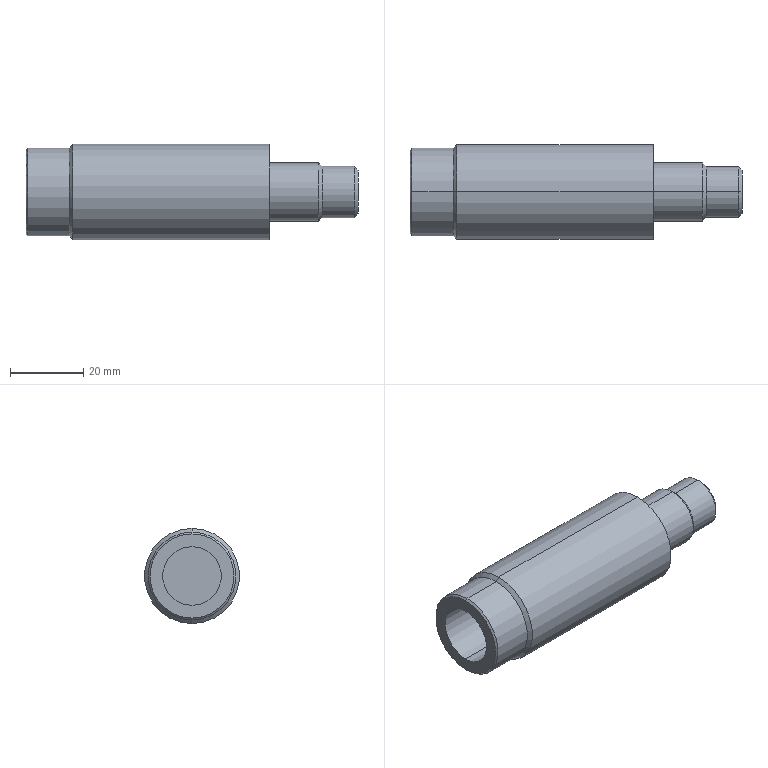Part | SolidWorks | features Chamfer 3, Revolution 1 | 1 solid | 22 faces | box 90.69 x 26 x 26 mm | volume 34532 mm3 | cylinder 10 | cone 8 | plane 4 | commonest cylinder face diameters 16 x4 14 x2 24 x2 26 x2
STEP:
#1=CARTESIAN_POINT('',(-33.026,0.,11.5));
#2=VERTEX_POINT('',#1);
#3=CARTESIAN_POINT('',(-33.026,0.,-11.5));
#4=VERTEX_POINT('',#3);
#5=CARTESIAN_POINT('',(-33.026,0.,0.));
#6=DIRECTION('',(-1.,0.,0.));
#7=DIRECTION('',(0.,0.,-1.));
#8=AXIS2_PLACEMENT_3D('',#5,#6,#7);
#9=CIRCLE('',#8,11.5);
#10=EDGE_CURVE('',#2,#4,#9,.T.);
#11=ORIENTED_EDGE('',*,*,#10,.F.);
#12=CARTESIAN_POINT('',(-32.526,0.,12.));
#13=VERTEX_POINT('',#12);
#14=CARTESIAN_POINT('',(-33.026,0.,11.5));
#15=DIRECTION('',(0.7071,0.,0.7071));
#16=VECTOR('',#15,1000.);
#17=LINE('',#14,#16);
#18=EDGE_CURVE('',#2,#13,#17,.T.);
#19=ORIENTED_EDGE('',*,*,#18,.T.);
#20=CARTESIAN_POINT('',(-32.526,0.,-12.));
#21=VERTEX_POINT('',#20);
#22=CARTESIAN_POINT('',(-32.526,0.,0.));
#23=DIRECTION('',(1.,0.,0.));
#24=DIRECTION('',(0.,0.,-1.));
#25=AXIS2_PLACEMENT_3D('',#22,#23,#24);
#26=CIRCLE('',#25,12.);
#27=EDGE_CURVE('',#21,#13,#26,.T.);
#28=ORIENTED_EDGE('',*,*,#27,.F.);
#29=CARTESIAN_POINT('',(-33.026,0.,-11.5));
#30=DIRECTION('',(0.7071,0.,-0.7071));
#31=VECTOR('',#30,1000.);
#32=LINE('',#29,#31);
#33=EDGE_CURVE('',#4,#21,#32,.T.);
#34=ORIENTED_EDGE('',*,*,#33,.F.);
#35=EDGE_LOOP('',(#11,#19,#28,#34));
#36=FACE_OUTER_BOUND('',#35,.T.);
#37=CARTESIAN_POINT('',(-33.026,0.,0.));
#38=DIRECTION('',(1.,0.,0.));
#39=DIRECTION('',(0.,0.,-1.));
#40=AXIS2_PLACEMENT_3D('',#37,#38,#39);
#41=CONICAL_SURFACE('',#40,11.5,0.7854);
#42=ADVANCED_FACE('',(#36),#41,.T.);
#43=CARTESIAN_POINT('',(47.874,0.,7.));
#44=VERTEX_POINT('',#43);
#45=CARTESIAN_POINT('',(47.874,0.,-7.));
#46=VERTEX_POINT('',#45);
#47=CARTESIAN_POINT('',(47.874,0.,0.));
#48=DIRECTION('',(-1.,0.,0.));
#49=DIRECTION('',(0.,0.,1.));
#50=AXIS2_PLACEMENT_3D('',#47,#48,#49);
#51=CIRCLE('',#50,7.);
#52=EDGE_CURVE('',#44,#46,#51,.T.);
#53=ORIENTED_EDGE('',*,*,#52,.T.);
#54=CARTESIAN_POINT('',(46.874,0.,-8.));
#55=VERTEX_POINT('',#54);
#56=CARTESIAN_POINT('',(46.874,0.,-8.));
#57=DIRECTION('',(-0.7071,0.,-0.7071));
#58=VECTOR('',#57,1000.);
#59=LINE('',#56,#58);
#60=EDGE_CURVE('',#46,#55,#59,.T.);
#61=ORIENTED_EDGE('',*,*,#60,.T.);
#62=CARTESIAN_POINT('',(46.874,0.,8.));
#63=VERTEX_POINT('',#62);
#64=CARTESIAN_POINT('',(46.874,0.,0.));
#65=DIRECTION('',(-1.,0.,0.));
#66=DIRECTION('',(0.,0.,1.));
#67=AXIS2_PLACEMENT_3D('',#64,#65,#66);
#68=CIRCLE('',#67,8.);
#69=EDGE_CURVE('',#63,#55,#68,.T.);
#70=ORIENTED_EDGE('',*,*,#69,.F.);
#71=CARTESIAN_POINT('',(46.874,0.,8.));
#72=DIRECTION('',(-0.7071,0.,0.7071));
#73=VECTOR('',#72,1000.);
#74=LINE('',#71,#73);
#75=EDGE_CURVE('',#44,#63,#74,.T.);
#76=ORIENTED_EDGE('',*,*,#75,.F.);
#77=EDGE_LOOP('',(#53,#61,#70,#76));
#78=FACE_OUTER_BOUND('',#77,.T.);
#79=CARTESIAN_POINT('',(46.874,0.,0.));
#80=DIRECTION('',(-1.,0.,0.));
#81=DIRECTION('',(0.,0.,1.));
#82=AXIS2_PLACEMENT_3D('',#79,#80,#81);
#83=CONICAL_SURFACE('',#82,8.,0.7854);
#84=ADVANCED_FACE('',(#78),#83,.T.);
#85=CARTESIAN_POINT('',(57.664,0.,-6.));
#86=VERTEX_POINT('',#85);
#87=CARTESIAN_POINT('',(57.664,0.,6.));
#88=VERTEX_POINT('',#87);
#89=CARTESIAN_POINT('',(57.664,0.,0.));
#90=DIRECTION('',(1.,0.,0.));
#91=DIRECTION('',(0.,0.,1.));
#92=AXIS2_PLACEMENT_3D('',#89,#90,#91);
#93=CIRCLE('',#92,6.);
#94=EDGE_CURVE('',#86,#88,#93,.T.);
#95=ORIENTED_EDGE('',*,*,#94,.F.);
#96=CARTESIAN_POINT('',(56.664,0.,-7.));
#97=VERTEX_POINT('',#96);
#98=CARTESIAN_POINT('',(56.664,0.,-7.));
#99=DIRECTION('',(-0.7071,0.,-0.7071));
#100=VECTOR('',#99,1000.);
#101=LINE('',#98,#100);
#102=EDGE_CURVE('',#86,#97,#101,.T.);
#103=ORIENTED_EDGE('',*,*,#102,.T.);
#104=CARTESIAN_POINT('',(56.664,0.,7.));
#105=VERTEX_POINT('',#104);
#106=CARTESIAN_POINT('',(56.664,0.,0.));
#107=DIRECTION('',(-1.,0.,0.));
#108=DIRECTION('',(0.,0.,1.));
#109=AXIS2_PLACEMENT_3D('',#106,#107,#108);
#110=CIRCLE('',#109,7.);
#111=EDGE_CURVE('',#105,#97,#110,.T.);
#112=ORIENTED_EDGE('',*,*,#111,.F.);
#113=CARTESIAN_POINT('',(56.664,0.,7.));
#114=DIRECTION('',(-0.7071,0.,0.7071));
#115=VECTOR('',#114,1000.);
#116=LINE('',#113,#115);
#117=EDGE_CURVE('',#88,#105,#116,.T.);
#118=ORIENTED_EDGE('',*,*,#117,.F.);
#119=EDGE_LOOP('',(#95,#103,#112,#118));
#120=FACE_OUTER_BOUND('',#119,.T.);
#121=CARTESIAN_POINT('',(56.664,0.,0.));
#122=DIRECTION('',(-1.,0.,0.));
#123=DIRECTION('',(0.,0.,1.));
#124=AXIS2_PLACEMENT_3D('',#121,#122,#123);
#125=CONICAL_SURFACE('',#124,7.,0.7854);
#126=ADVANCED_FACE('',(#120),#125,.T.);
#127=CARTESIAN_POINT('',(-21.21,0.,12.));
#128=VERTEX_POINT('',#127);
#129=CARTESIAN_POINT('',(-21.21,0.,-12.));
#130=VERTEX_POINT('',#129);
#131=CARTESIAN_POINT('',(-21.21,0.,0.));
#132=DIRECTION('',(-1.,0.,0.));
#133=DIRECTION('',(0.,0.,1.));
#134=AXIS2_PLACEMENT_3D('',#131,#132,#133);
#135=CIRCLE('',#134,12.);
#136=EDGE_CURVE('',#128,#130,#135,.T.);
#137=ORIENTED_EDGE('',*,*,#136,.F.);
#138=CARTESIAN_POINT('',(-20.21,0.,13.));
#139=VERTEX_POINT('',#138);
#140=CARTESIAN_POINT('',(-21.21,0.,12.));
#141=DIRECTION('',(0.7071,0.,0.7071));
#142=VECTOR('',#141,1000.);
#143=LINE('',#140,#142);
#144=EDGE_CURVE('',#128,#139,#143,.T.);
#145=ORIENTED_EDGE('',*,*,#144,.T.);
#146=CARTESIAN_POINT('',(-20.21,0.,-13.));
#147=VERTEX_POINT('',#146);
#148=CARTESIAN_POINT('',(-20.21,0.,0.));
#149=DIRECTION('',(1.,0.,0.));
#150=DIRECTION('',(0.,0.,-1.));
#151=AXIS2_PLACEMENT_3D('',#148,#149,#150);
#152=CIRCLE('',#151,13.);
#153=EDGE_CURVE('',#147,#139,#152,.T.);
#154=ORIENTED_EDGE('',*,*,#153,.F.);
#155=CARTESIAN_POINT('',(-21.21,0.,-12.));
#156=DIRECTION('',(0.7071,0.,-0.7071));
#157=VECTOR('',#156,1000.);
#158=LINE('',#155,#157);
#159=EDGE_CURVE('',#130,#147,#158,.T.);
#160=ORIENTED_EDGE('',*,*,#159,.F.);
#161=EDGE_LOOP('',(#137,#145,#154,#160));
#162=FACE_OUTER_BOUND('',#161,.T.);
#163=CARTESIAN_POINT('',(-21.21,0.,0.));
#164=DIRECTION('',(1.,0.,0.));
#165=DIRECTION('',(0.,0.,-1.));
#166=AXIS2_PLACEMENT_3D('',#163,#164,#165);
#167=CONICAL_SURFACE('',#166,12.,0.7854);
#168=ADVANCED_FACE('',(#162),#167,.T.);
#169=ORIENTED_EDGE('',*,*,#111,.T.);
#170=CARTESIAN_POINT('',(-58.891,0.,-7.));
#171=DIRECTION('',(-1.,0.,0.));
#172=VECTOR('',#171,1000.);
#173=LINE('',#170,#172);
#174=EDGE_CURVE('',#97,#46,#173,.T.);
#175=ORIENTED_EDGE('',*,*,#174,.T.);
#176=ORIENTED_EDGE('',*,*,#52,.F.);
#177=CARTESIAN_POINT('',(-58.891,0.,7.));
#178=DIRECTION('',(-1.,0.,0.));
#179=VECTOR('',#178,1000.);
#180=LINE('',#177,#179);
#181=EDGE_CURVE('',#105,#44,#180,.T.);
#182=ORIENTED_EDGE('',*,*,#181,.F.);
#183=EDGE_LOOP('',(#169,#175,#176,#182));
#184=FACE_OUTER_BOUND('',#183,.T.);
#185=CARTESIAN_POINT('',(-58.891,0.,0.));
#186=DIRECTION('',(-1.,0.,0.));
#187=DIRECTION('',(0.,0.,1.));
#188=AXIS2_PLACEMENT_3D('',#185,#186,#187);
#189=CYLINDRICAL_SURFACE('',#188,7.);
#190=ADVANCED_FACE('',(#184),#189,.T.);
#191=ORIENTED_EDGE('',*,*,#69,.T.);
#192=CARTESIAN_POINT('',(33.374,0.,-8.));
#193=VERTEX_POINT('',#192);
#194=CARTESIAN_POINT('',(-58.891,0.,-8.));
#195=DIRECTION('',(-1.,0.,0.));
#196=VECTOR('',#195,1000.);
#197=LINE('',#194,#196);
#198=EDGE_CURVE('',#55,#193,#197,.T.);
#199=ORIENTED_EDGE('',*,*,#198,.T.);
#200=CARTESIAN_POINT('',(33.374,0.,8.));
#201=VERTEX_POINT('',#200);
#202=CARTESIAN_POINT('',(33.374,0.,0.));
#203=DIRECTION('',(-1.,0.,0.));
#204=DIRECTION('',(0.,0.,1.));
#205=AXIS2_PLACEMENT_3D('',#202,#203,#204);
#206=CIRCLE('',#205,8.);
#207=EDGE_CURVE('',#201,#193,#206,.T.);
#208=ORIENTED_EDGE('',*,*,#207,.F.);
#209=CARTESIAN_POINT('',(-58.891,0.,8.));
#210=DIRECTION('',(-1.,0.,0.));
#211=VECTOR('',#210,1000.);
#212=LINE('',#209,#211);
#213=EDGE_CURVE('',#63,#201,#212,.T.);
#214=ORIENTED_EDGE('',*,*,#213,.F.);
#215=EDGE_LOOP('',(#191,#199,#208,#214));
#216=FACE_OUTER_BOUND('',#215,.T.);
#217=CARTESIAN_POINT('',(-58.891,0.,0.));
#218=DIRECTION('',(-1.,0.,0.));
#219=DIRECTION('',(0.,0.,1.));
#220=AXIS2_PLACEMENT_3D('',#217,#218,#219);
#221=CYLINDRICAL_SURFACE('',#220,8.);
#222=ADVANCED_FACE('',(#216),#221,.T.);
#223=CARTESIAN_POINT('',(33.374,0.,13.));
#224=VERTEX_POINT('',#223);
#225=CARTESIAN_POINT('',(33.374,0.,-13.));
#226=VERTEX_POINT('',#225);
#227=CARTESIAN_POINT('',(33.374,0.,0.));
#228=DIRECTION('',(-1.,0.,0.));
#229=DIRECTION('',(0.,0.,1.));
#230=AXIS2_PLACEMENT_3D('',#227,#228,#229);
#231=CIRCLE('',#230,13.);
#232=EDGE_CURVE('',#224,#226,#231,.T.);
#233=ORIENTED_EDGE('',*,*,#232,.T.);
#234=CARTESIAN_POINT('',(-58.891,0.,-13.));
#235=DIRECTION('',(-1.,0.,0.));
#236=VECTOR('',#235,1000.);
#237=LINE('',#234,#236);
#238=EDGE_CURVE('',#226,#147,#237,.T.);
#239=ORIENTED_EDGE('',*,*,#238,.T.);
#240=ORIENTED_EDGE('',*,*,#153,.T.);
#241=CARTESIAN_POINT('',(-58.891,0.,13.));
#242=DIRECTION('',(-1.,0.,0.));
#243=VECTOR('',#242,1000.);
#244=LINE('',#241,#243);
#245=EDGE_CURVE('',#224,#139,#244,.T.);
#246=ORIENTED_EDGE('',*,*,#245,.F.);
#247=EDGE_LOOP('',(#233,#239,#240,#246));
#248=FACE_OUTER_BOUND('',#247,.T.);
#249=CARTESIAN_POINT('',(-58.891,0.,0.));
#250=DIRECTION('',(-1.,0.,0.));
#251=DIRECTION('',(0.,0.,1.));
#252=AXIS2_PLACEMENT_3D('',#249,#250,#251);
#253=CYLINDRICAL_SURFACE('',#252,13.);
#254=ADVANCED_FACE('',(#248),#253,.T.);
#255=ORIENTED_EDGE('',*,*,#136,.T.);
#256=CARTESIAN_POINT('',(-58.891,0.,-12.));
#257=DIRECTION('',(-1.,0.,0.));
#258=VECTOR('',#257,1000.);
#259=LINE('',#256,#258);
#260=EDGE_CURVE('',#130,#21,#259,.T.);
#261=ORIENTED_EDGE('',*,*,#260,.T.);
#262=ORIENTED_EDGE('',*,*,#27,.T.);
#263=CARTESIAN_POINT('',(-58.891,0.,12.));
#264=DIRECTION('',(-1.,0.,0.));
#265=VECTOR('',#264,1000.);
#266=LINE('',#263,#265);
#267=EDGE_CURVE('',#128,#13,#266,.T.);
#268=ORIENTED_EDGE('',*,*,#267,.F.);
#269=EDGE_LOOP('',(#255,#261,#262,#268));
#270=FACE_OUTER_BOUND('',#269,.T.);
#271=CARTESIAN_POINT('',(-58.891,0.,0.));
#272=DIRECTION('',(-1.,0.,0.));
#273=DIRECTION('',(0.,0.,1.));
#274=AXIS2_PLACEMENT_3D('',#271,#272,#273);
#275=CYLINDRICAL_SURFACE('',#274,12.);
#276=ADVANCED_FACE('',(#270),#275,.T.);
#277=CARTESIAN_POINT('',(-12.526,0.,-8.));
#278=VERTEX_POINT('',#277);
#279=CARTESIAN_POINT('',(-12.526,0.,8.));
#280=VERTEX_POINT('',#279);
#281=CARTESIAN_POINT('',(-12.526,0.,0.));
#282=DIRECTION('',(-1.,0.,0.));
#283=DIRECTION('',(0.,0.,1.));
#284=AXIS2_PLACEMENT_3D('',#281,#282,#283);
#285=CIRCLE('',#284,8.);
#286=EDGE_CURVE('',#278,#280,#285,.T.);
#287=ORIENTED_EDGE('',*,*,#286,.F.);
#288=CARTESIAN_POINT('',(-33.026,0.,-8.));
#289=VERTEX_POINT('',#288);
#290=CARTESIAN_POINT('',(-58.891,0.,-8.));
#291=DIRECTION('',(-1.,0.,0.));
#292=VECTOR('',#291,1000.);
#293=LINE('',#290,#292);
#294=EDGE_CURVE('',#278,#289,#293,.T.);
#295=ORIENTED_EDGE('',*,*,#294,.T.);
#296=CARTESIAN_POINT('',(-33.026,0.,8.));
#297=VERTEX_POINT('',#296);
#298=CARTESIAN_POINT('',(-33.026,0.,0.));
#299=DIRECTION('',(-1.,0.,0.));
#300=DIRECTION('',(0.,0.,1.));
#301=AXIS2_PLACEMENT_3D('',#298,#299,#300);
#302=CIRCLE('',#301,8.);
#303=EDGE_CURVE('',#289,#297,#302,.T.);
#304=ORIENTED_EDGE('',*,*,#303,.T.);
#305=CARTESIAN_POINT('',(-58.891,0.,8.));
#306=DIRECTION('',(-1.,0.,0.));
#307=VECTOR('',#306,1000.);
#308=LINE('',#305,#307);
#309=EDGE_CURVE('',#280,#297,#308,.T.);
#310=ORIENTED_EDGE('',*,*,#309,.F.);
#311=EDGE_LOOP('',(#287,#295,#304,#310));
#312=FACE_OUTER_BOUND('',#311,.T.);
#313=CARTESIAN_POINT('',(-58.891,0.,0.));
#314=DIRECTION('',(-1.,0.,0.));
#315=DIRECTION('',(0.,0.,1.));
#316=AXIS2_PLACEMENT_3D('',#313,#314,#315);
#317=CYLINDRICAL_SURFACE('',#316,8.);
#318=ADVANCED_FACE('',(#312),#317,.F.);
#319=ORIENTED_EDGE('',*,*,#294,.F.);
#320=CARTESIAN_POINT('',(-12.526,0.,0.));
#321=DIRECTION('',(-1.,0.,0.));
#322=DIRECTION('',(0.,0.,1.));
#323=AXIS2_PLACEMENT_3D('',#320,#321,#322);
#324=CIRCLE('',#323,8.);
#325=EDGE_CURVE('',#280,#278,#324,.T.);
#326=ORIENTED_EDGE('',*,*,#325,.F.);
#327=ORIENTED_EDGE('',*,*,#309,.T.);
#328=CARTESIAN_POINT('',(-33.026,0.,0.));
#329=DIRECTION('',(-1.,0.,0.));
#330=DIRECTION('',(0.,0.,1.));
#331=AXIS2_PLACEMENT_3D('',#328,#329,#330);
#332=CIRCLE('',#331,8.);
#333=EDGE_CURVE('',#297,#289,#332,.T.);
#334=ORIENTED_EDGE('',*,*,#333,.T.);
#335=EDGE_LOOP('',(#319,#326,#327,#334));
#336=FACE_OUTER_BOUND('',#335,.T.);
#337=CARTESIAN_POINT('',(-58.891,0.,0.));
#338=DIRECTION('',(-1.,0.,0.));
#339=DIRECTION('',(0.,0.,1.));
#340=AXIS2_PLACEMENT_3D('',#337,#338,#339);
#341=CYLINDRICAL_SURFACE('',#340,8.);
#342=ADVANCED_FACE('',(#336),#341,.F.);
#343=CARTESIAN_POINT('',(-33.026,0.,0.));
#344=DIRECTION('',(-1.,0.,0.));
#345=DIRECTION('',(0.,0.,-1.));
#346=AXIS2_PLACEMENT_3D('',#343,#344,#345);
#347=CIRCLE('',#346,11.5);
#348=EDGE_CURVE('',#4,#2,#347,.T.);
#349=ORIENTED_EDGE('',*,*,#348,.T.);
#350=ORIENTED_EDGE('',*,*,#10,.T.);
#351=EDGE_LOOP('',(#349,#350));
#352=FACE_OUTER_BOUND('',#351,.T.);
#353=ORIENTED_EDGE('',*,*,#333,.F.);
#354=ORIENTED_EDGE('',*,*,#303,.F.);
#355=EDGE_LOOP('',(#353,#354));
#356=FACE_BOUND('',#355,.T.);
#357=CARTESIAN_POINT('',(-33.026,8.,0.));
#358=DIRECTION('',(1.,0.,0.));
#359=DIRECTION('',(0.,0.,-1.));
#360=AXIS2_PLACEMENT_3D('',#357,#358,#359);
#361=PLANE('',#360);
#362=ADVANCED_FACE('',(#352,#356),#361,.F.);
#363=ORIENTED_EDGE('',*,*,#260,.F.);
#364=CARTESIAN_POINT('',(-21.21,0.,0.));
#365=DIRECTION('',(-1.,0.,0.));
#366=DIRECTION('',(0.,0.,1.));
#367=AXIS2_PLACEMENT_3D('',#364,#365,#366);
#368=CIRCLE('',#367,12.);
#369=EDGE_CURVE('',#130,#128,#368,.T.);
#370=ORIENTED_EDGE('',*,*,#369,.T.);
#371=ORIENTED_EDGE('',*,*,#267,.T.);
#372=CARTESIAN_POINT('',(-32.526,0.,0.));
#373=DIRECTION('',(1.,0.,0.));
#374=DIRECTION('',(0.,0.,-1.));
#375=AXIS2_PLACEMENT_3D('',#372,#373,#374);
#376=CIRCLE('',#375,12.);
#377=EDGE_CURVE('',#13,#21,#376,.T.);
#378=ORIENTED_EDGE('',*,*,#377,.T.);
#379=EDGE_LOOP('',(#363,#370,#371,#378));
#380=FACE_OUTER_BOUND('',#379,.T.);
#381=CARTESIAN_POINT('',(-58.891,0.,0.));
#382=DIRECTION('',(-1.,0.,0.));
#383=DIRECTION('',(0.,0.,1.));
#384=AXIS2_PLACEMENT_3D('',#381,#382,#383);
#385=CYLINDRICAL_SURFACE('',#384,12.);
#386=ADVANCED_FACE('',(#380),#385,.T.);
#387=ORIENTED_EDGE('',*,*,#238,.F.);
#388=CARTESIAN_POINT('',(33.374,0.,0.));
#389=DIRECTION('',(-1.,0.,0.));
#390=DIRECTION('',(0.,0.,1.));
#391=AXIS2_PLACEMENT_3D('',#388,#389,#390);
#392=CIRCLE('',#391,13.);
#393=EDGE_CURVE('',#226,#224,#392,.T.);
#394=ORIENTED_EDGE('',*,*,#393,.T.);
#395=ORIENTED_EDGE('',*,*,#245,.T.);
#396=CARTESIAN_POINT('',(-20.21,0.,0.));
#397=DIRECTION('',(1.,0.,0.));
#398=DIRECTION('',(0.,0.,-1.));
#399=AXIS2_PLACEMENT_3D('',#396,#397,#398);
#400=CIRCLE('',#399,13.);
#401=EDGE_CURVE('',#139,#147,#400,.T.);
#402=ORIENTED_EDGE('',*,*,#401,.T.);
#403=EDGE_LOOP('',(#387,#394,#395,#402));
#404=FACE_OUTER_BOUND('',#403,.T.);
#405=CARTESIAN_POINT('',(-58.891,0.,0.));
#406=DIRECTION('',(-1.,0.,0.));
#407=DIRECTION('',(0.,0.,1.));
#408=AXIS2_PLACEMENT_3D('',#405,#406,#407);
#409=CYLINDRICAL_SURFACE('',#408,13.);
#410=ADVANCED_FACE('',(#404),#409,.T.);
#411=ORIENTED_EDGE('',*,*,#232,.F.);
#412=ORIENTED_EDGE('',*,*,#393,.F.);
#413=EDGE_LOOP('',(#411,#412));
#414=FACE_OUTER_BOUND('',#413,.T.);
#415=ORIENTED_EDGE('',*,*,#207,.T.);
#416=CARTESIAN_POINT('',(33.374,0.,0.));
#417=DIRECTION('',(-1.,0.,0.));
#418=DIRECTION('',(0.,0.,1.));
#419=AXIS2_PLACEMENT_3D('',#416,#417,#418);
#420=CIRCLE('',#419,8.);
#421=EDGE_CURVE('',#193,#201,#420,.T.);
#422=ORIENTED_EDGE('',*,*,#421,.T.);
#423=EDGE_LOOP('',(#415,#422));
#424=FACE_BOUND('',#423,.T.);
#425=CARTESIAN_POINT('',(33.374,13.,0.));
#426=DIRECTION('',(-1.,0.,0.));
#427=DIRECTION('',(0.,0.,1.));
#428=AXIS2_PLACEMENT_3D('',#425,#426,#427);
#429=PLANE('',#428);
#430=ADVANCED_FACE('',(#414,#424),#429,.F.);
#431=ORIENTED_EDGE('',*,*,#198,.F.);
#432=CARTESIAN_POINT('',(46.874,0.,0.));
#433=DIRECTION('',(-1.,0.,0.));
#434=DIRECTION('',(0.,0.,1.));
#435=AXIS2_PLACEMENT_3D('',#432,#433,#434);
#436=CIRCLE('',#435,8.);
#437=EDGE_CURVE('',#55,#63,#436,.T.);
#438=ORIENTED_EDGE('',*,*,#437,.T.);
#439=ORIENTED_EDGE('',*,*,#213,.T.);
#440=ORIENTED_EDGE('',*,*,#421,.F.);
#441=EDGE_LOOP('',(#431,#438,#439,#440));
#442=FACE_OUTER_BOUND('',#441,.T.);
#443=CARTESIAN_POINT('',(-58.891,0.,0.));
#444=DIRECTION('',(-1.,0.,0.));
#445=DIRECTION('',(0.,0.,1.));
#446=AXIS2_PLACEMENT_3D('',#443,#444,#445);
#447=CYLINDRICAL_SURFACE('',#446,8.);
#448=ADVANCED_FACE('',(#442),#447,.T.);
#449=ORIENTED_EDGE('',*,*,#174,.F.);
#450=CARTESIAN_POINT('',(56.664,0.,0.));
#451=DIRECTION('',(-1.,0.,0.));
#452=DIRECTION('',(0.,0.,1.));
#453=AXIS2_PLACEMENT_3D('',#450,#451,#452);
#454=CIRCLE('',#453,7.);
#455=EDGE_CURVE('',#97,#105,#454,.T.);
#456=ORIENTED_EDGE('',*,*,#455,.T.);
#457=ORIENTED_EDGE('',*,*,#181,.T.);
#458=CARTESIAN_POINT('',(47.874,0.,0.));
#459=DIRECTION('',(-1.,0.,0.));
#460=DIRECTION('',(0.,0.,1.));
#461=AXIS2_PLACEMENT_3D('',#458,#459,#460);
#462=CIRCLE('',#461,7.);
#463=EDGE_CURVE('',#46,#44,#462,.T.);
#464=ORIENTED_EDGE('',*,*,#463,.F.);
#465=EDGE_LOOP('',(#449,#456,#457,#464));
#466=FACE_OUTER_BOUND('',#465,.T.);
#467=CARTESIAN_POINT('',(-58.891,0.,0.));
#468=DIRECTION('',(-1.,0.,0.));
#469=DIRECTION('',(0.,0.,1.));
#470=AXIS2_PLACEMENT_3D('',#467,#468,#469);
#471=CYLINDRICAL_SURFACE('',#470,7.);
#472=ADVANCED_FACE('',(#466),#471,.T.);
#473=CARTESIAN_POINT('',(57.664,0.,0.));
#474=DIRECTION('',(1.,0.,0.));
#475=DIRECTION('',(0.,0.,1.));
#476=AXIS2_PLACEMENT_3D('',#473,#474,#475);
#477=CIRCLE('',#476,6.);
#478=EDGE_CURVE('',#88,#86,#477,.T.);
#479=ORIENTED_EDGE('',*,*,#478,.T.);
#480=ORIENTED_EDGE('',*,*,#94,.T.);
#481=EDGE_LOOP('',(#479,#480));
#482=FACE_OUTER_BOUND('',#481,.T.);
#483=CARTESIAN_POINT('',(57.664,7.,0.));
#484=DIRECTION('',(-1.,0.,0.));
#485=DIRECTION('',(0.,0.,1.));
#486=AXIS2_PLACEMENT_3D('',#483,#484,#485);
#487=PLANE('',#486);
#488=ADVANCED_FACE('',(#482),#487,.F.);
#489=ORIENTED_EDGE('',*,*,#325,.T.);
#490=ORIENTED_EDGE('',*,*,#286,.T.);
#491=EDGE_LOOP('',(#489,#490));
#492=FACE_OUTER_BOUND('',#491,.T.);
#493=CARTESIAN_POINT('',(-12.526,0.,0.));
#494=DIRECTION('',(1.,0.,0.));
#495=DIRECTION('',(0.,0.,-1.));
#496=AXIS2_PLACEMENT_3D('',#493,#494,#495);
#497=PLANE('',#496);
#498=ADVANCED_FACE('',(#492),#497,.F.);
#499=ORIENTED_EDGE('',*,*,#144,.F.);
#500=ORIENTED_EDGE('',*,*,#369,.F.);
#501=ORIENTED_EDGE('',*,*,#159,.T.);
#502=ORIENTED_EDGE('',*,*,#401,.F.);
#503=EDGE_LOOP('',(#499,#500,#501,#502));
#504=FACE_OUTER_BOUND('',#503,.T.);
#505=CARTESIAN_POINT('',(-21.21,0.,0.));
#506=DIRECTION('',(1.,0.,0.));
#507=DIRECTION('',(0.,0.,-1.));
#508=AXIS2_PLACEMENT_3D('',#505,#506,#507);
#509=CONICAL_SURFACE('',#508,12.,0.7854);
#510=ADVANCED_FACE('',(#504),#509,.T.);
#511=ORIENTED_EDGE('',*,*,#102,.F.);
#512=ORIENTED_EDGE('',*,*,#478,.F.);
#513=ORIENTED_EDGE('',*,*,#117,.T.);
#514=ORIENTED_EDGE('',*,*,#455,.F.);
#515=EDGE_LOOP('',(#511,#512,#513,#514));
#516=FACE_OUTER_BOUND('',#515,.T.);
#517=CARTESIAN_POINT('',(56.664,0.,0.));
#518=DIRECTION('',(-1.,0.,0.));
#519=DIRECTION('',(0.,0.,1.));
#520=AXIS2_PLACEMENT_3D('',#517,#518,#519);
#521=CONICAL_SURFACE('',#520,7.,0.7854);
#522=ADVANCED_FACE('',(#516),#521,.T.);
#523=ORIENTED_EDGE('',*,*,#60,.F.);
#524=ORIENTED_EDGE('',*,*,#463,.T.);
#525=ORIENTED_EDGE('',*,*,#75,.T.);
#526=ORIENTED_EDGE('',*,*,#437,.F.);
#527=EDGE_LOOP('',(#523,#524,#525,#526));
#528=FACE_OUTER_BOUND('',#527,.T.);
#529=CARTESIAN_POINT('',(46.874,0.,0.));
#530=DIRECTION('',(-1.,0.,0.));
#531=DIRECTION('',(0.,0.,1.));
#532=AXIS2_PLACEMENT_3D('',#529,#530,#531);
#533=CONICAL_SURFACE('',#532,8.,0.7854);
#534=ADVANCED_FACE('',(#528),#533,.T.);
#535=ORIENTED_EDGE('',*,*,#18,.F.);
#536=ORIENTED_EDGE('',*,*,#348,.F.);
#537=ORIENTED_EDGE('',*,*,#33,.T.);
#538=ORIENTED_EDGE('',*,*,#377,.F.);
#539=EDGE_LOOP('',(#535,#536,#537,#538));
#540=FACE_OUTER_BOUND('',#539,.T.);
#541=CARTESIAN_POINT('',(-33.026,0.,0.));
#542=DIRECTION('',(1.,0.,0.));
#543=DIRECTION('',(0.,0.,-1.));
#544=AXIS2_PLACEMENT_3D('',#541,#542,#543);
#545=CONICAL_SURFACE('',#544,11.5,0.7854);
#546=ADVANCED_FACE('',(#540),#545,.T.);
#547=CLOSED_SHELL('',(#42,#84,#126,#168,#190,#222,#254,#276,#318,#342,#362,#386,#410,#430,#448,#472,#488,#498,#510,#522,#534,#546));
#548=MANIFOLD_SOLID_BREP('',#547);
#549=CARTESIAN_POINT('',(0.,0.,0.));
#550=DIRECTION('',(0.,0.,1.));
#551=DIRECTION('',(1.,0.,0.));
#552=AXIS2_PLACEMENT_3D('',#549,#550,#551);
#553=(LENGTH_UNIT()NAMED_UNIT(*)SI_UNIT(.MILLI.,.METRE.));
#554=UNCERTAINTY_MEASURE_WITH_UNIT(LENGTH_MEASURE(0.00001),#553,'','');
#555=(NAMED_UNIT(*)PLANE_ANGLE_UNIT()SI_UNIT($,.RADIAN.));
#556=(NAMED_UNIT(*)SI_UNIT($,.STERADIAN.)SOLID_ANGLE_UNIT());
#557=(GEOMETRIC_REPRESENTATION_CONTEXT(3)GLOBAL_UNCERTAINTY_ASSIGNED_CONTEXT((#554))GLOBAL_UNIT_ASSIGNED_CONTEXT((#553,#555,#556))REPRESENTATION_CONTEXT('',''));
#558=ADVANCED_BREP_SHAPE_REPRESENTATION('',(#548,#552),#557);